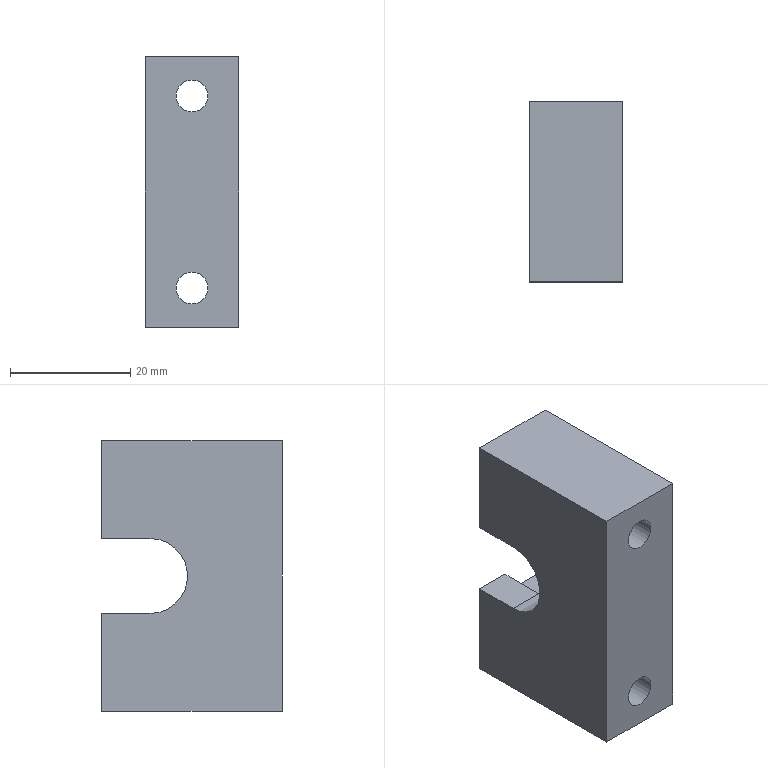Part | NX | 1 solid | 20 faces | box 15.5 x 30 x 45 mm | volume 14039 mm3 | plane 14 | cylinder 6 | commonest cylinder face diameters 5.3 x2 10 x2 12.5 x1 20 x1
STEP:
#1=CARTESIAN_POINT('',(6.,7.,-6.25));
#2=VERTEX_POINT('',#1);
#3=CARTESIAN_POINT('',(6.,7.,6.25));
#4=VERTEX_POINT('',#3);
#5=CARTESIAN_POINT('',(6.,7.,0.));
#6=DIRECTION('',(1.,0.,0.));
#7=DIRECTION('',(0.,0.,-1.));
#8=AXIS2_PLACEMENT_3D('',#5,#6,#7);
#9=CIRCLE('',#8,6.25);
#10=EDGE_CURVE('',#2,#4,#9,.F.);
#11=ORIENTED_EDGE('',*,*,#10,.F.);
#12=CARTESIAN_POINT('',(0.,7.,-6.25));
#13=VERTEX_POINT('',#12);
#14=CARTESIAN_POINT('',(-4.5,7.,-6.25));
#15=DIRECTION('',(1.,0.,0.));
#16=VECTOR('',#15,1000.);
#17=LINE('',#14,#16);
#18=EDGE_CURVE('',#13,#2,#17,.T.);
#19=ORIENTED_EDGE('',*,*,#18,.F.);
#20=CARTESIAN_POINT('',(0.,7.,6.25));
#21=VERTEX_POINT('',#20);
#22=CARTESIAN_POINT('',(0.,7.,0.));
#23=DIRECTION('',(1.,0.,0.));
#24=DIRECTION('',(0.,0.,-1.));
#25=AXIS2_PLACEMENT_3D('',#22,#23,#24);
#26=CIRCLE('',#25,6.25);
#27=EDGE_CURVE('',#21,#13,#26,.T.);
#28=ORIENTED_EDGE('',*,*,#27,.F.);
#29=CARTESIAN_POINT('',(-4.5,7.,6.25));
#30=DIRECTION('',(1.,0.,0.));
#31=VECTOR('',#30,1000.);
#32=LINE('',#29,#31);
#33=EDGE_CURVE('',#21,#4,#32,.T.);
#34=ORIENTED_EDGE('',*,*,#33,.T.);
#35=EDGE_LOOP('',(#11,#19,#28,#34));
#36=FACE_BOUND('',#35,.T.);
#37=CARTESIAN_POINT('',(-4.5,7.,0.));
#38=DIRECTION('',(1.,0.,0.));
#39=DIRECTION('',(0.,0.,-1.));
#40=AXIS2_PLACEMENT_3D('',#37,#38,#39);
#41=CYLINDRICAL_SURFACE('',#40,6.25);
#42=ADVANCED_FACE('',(#36),#41,.F.);
#43=CARTESIAN_POINT('',(6.,15.,6.25));
#44=VERTEX_POINT('',#43);
#45=CARTESIAN_POINT('',(6.,7.,6.25));
#46=DIRECTION('',(0.,1.,0.));
#47=VECTOR('',#46,1000.);
#48=LINE('',#45,#47);
#49=EDGE_CURVE('',#4,#44,#48,.T.);
#50=ORIENTED_EDGE('',*,*,#49,.F.);
#51=ORIENTED_EDGE('',*,*,#33,.F.);
#52=CARTESIAN_POINT('',(0.,15.,6.25));
#53=VERTEX_POINT('',#52);
#54=CARTESIAN_POINT('',(0.,0.,6.25));
#55=DIRECTION('',(0.,-1.,0.));
#56=VECTOR('',#55,1000.);
#57=LINE('',#54,#56);
#58=EDGE_CURVE('',#53,#21,#57,.T.);
#59=ORIENTED_EDGE('',*,*,#58,.F.);
#60=CARTESIAN_POINT('',(15.5,15.,6.25));
#61=DIRECTION('',(-1.,0.,0.));
#62=VECTOR('',#61,1000.);
#63=LINE('',#60,#62);
#64=EDGE_CURVE('',#44,#53,#63,.T.);
#65=ORIENTED_EDGE('',*,*,#64,.F.);
#66=EDGE_LOOP('',(#50,#51,#59,#65));
#67=FACE_BOUND('',#66,.T.);
#68=CARTESIAN_POINT('',(-4.5,7.,6.25));
#69=DIRECTION('',(0.,0.,1.));
#70=DIRECTION('',(0.,-1.,0.));
#71=AXIS2_PLACEMENT_3D('',#68,#69,#70);
#72=PLANE('',#71);
#73=ADVANCED_FACE('',(#67),#72,.F.);
#74=CARTESIAN_POINT('',(6.,15.,-6.25));
#75=VERTEX_POINT('',#74);
#76=CARTESIAN_POINT('',(6.,7.,-6.25));
#77=DIRECTION('',(0.,-1.,0.));
#78=VECTOR('',#77,1000.);
#79=LINE('',#76,#78);
#80=EDGE_CURVE('',#75,#2,#79,.T.);
#81=ORIENTED_EDGE('',*,*,#80,.F.);
#82=CARTESIAN_POINT('',(0.,15.,-6.25));
#83=VERTEX_POINT('',#82);
#84=CARTESIAN_POINT('',(15.5,15.,-6.25));
#85=DIRECTION('',(1.,0.,0.));
#86=VECTOR('',#85,1000.);
#87=LINE('',#84,#86);
#88=EDGE_CURVE('',#83,#75,#87,.T.);
#89=ORIENTED_EDGE('',*,*,#88,.F.);
#90=CARTESIAN_POINT('',(0.,0.,-6.25));
#91=DIRECTION('',(0.,1.,0.));
#92=VECTOR('',#91,1000.);
#93=LINE('',#90,#92);
#94=EDGE_CURVE('',#13,#83,#93,.T.);
#95=ORIENTED_EDGE('',*,*,#94,.F.);
#96=ORIENTED_EDGE('',*,*,#18,.T.);
#97=EDGE_LOOP('',(#81,#89,#95,#96));
#98=FACE_BOUND('',#97,.T.);
#99=CARTESIAN_POINT('',(-4.5,7.,-6.25));
#100=DIRECTION('',(0.,0.,-1.));
#101=DIRECTION('',(0.,1.,0.));
#102=AXIS2_PLACEMENT_3D('',#99,#100,#101);
#103=PLANE('',#102);
#104=ADVANCED_FACE('',(#98),#103,.F.);
#105=CARTESIAN_POINT('',(7.75,15.,21.));
#106=VERTEX_POINT('',#105);
#107=CARTESIAN_POINT('',(7.75,15.,16.));
#108=DIRECTION('',(0.,1.,0.));
#109=DIRECTION('',(0.,0.,1.));
#110=AXIS2_PLACEMENT_3D('',#107,#108,#109);
#111=CIRCLE('',#110,5.);
#112=EDGE_CURVE('',#106,#106,#111,.T.);
#113=ORIENTED_EDGE('',*,*,#112,.F.);
#114=EDGE_LOOP('',(#113));
#115=FACE_BOUND('',#114,.T.);
#116=CARTESIAN_POINT('',(15.5,15.,10.));
#117=VERTEX_POINT('',#116);
#118=CARTESIAN_POINT('',(15.5,15.,22.5));
#119=VERTEX_POINT('',#118);
#120=CARTESIAN_POINT('',(15.5,15.,22.5));
#121=DIRECTION('',(0.,0.,1.));
#122=VECTOR('',#121,1000.);
#123=LINE('',#120,#122);
#124=EDGE_CURVE('',#117,#119,#123,.T.);
#125=ORIENTED_EDGE('',*,*,#124,.F.);
#126=CARTESIAN_POINT('',(6.,15.,10.));
#127=VERTEX_POINT('',#126);
#128=CARTESIAN_POINT('',(6.,15.,10.));
#129=DIRECTION('',(1.,0.,0.));
#130=VECTOR('',#129,1000.);
#131=LINE('',#128,#130);
#132=EDGE_CURVE('',#127,#117,#131,.T.);
#133=ORIENTED_EDGE('',*,*,#132,.F.);
#134=CARTESIAN_POINT('',(6.,15.,22.5));
#135=DIRECTION('',(0.,0.,1.));
#136=VECTOR('',#135,1000.);
#137=LINE('',#134,#136);
#138=EDGE_CURVE('',#44,#127,#137,.T.);
#139=ORIENTED_EDGE('',*,*,#138,.F.);
#140=ORIENTED_EDGE('',*,*,#64,.T.);
#141=CARTESIAN_POINT('',(0.,15.,22.5));
#142=VERTEX_POINT('',#141);
#143=CARTESIAN_POINT('',(0.,15.,22.5));
#144=DIRECTION('',(0.,0.,1.));
#145=VECTOR('',#144,1000.);
#146=LINE('',#143,#145);
#147=EDGE_CURVE('',#53,#142,#146,.T.);
#148=ORIENTED_EDGE('',*,*,#147,.T.);
#149=CARTESIAN_POINT('',(15.5,15.,22.5));
#150=DIRECTION('',(-1.,0.,0.));
#151=VECTOR('',#150,1000.);
#152=LINE('',#149,#151);
#153=EDGE_CURVE('',#119,#142,#152,.T.);
#154=ORIENTED_EDGE('',*,*,#153,.F.);
#155=EDGE_LOOP('',(#125,#133,#139,#140,#148,#154));
#156=FACE_BOUND('',#155,.T.);
#157=CARTESIAN_POINT('',(15.5,15.,22.5));
#158=DIRECTION('',(0.,-1.,0.));
#159=DIRECTION('',(0.,0.,-1.));
#160=AXIS2_PLACEMENT_3D('',#157,#158,#159);
#161=PLANE('',#160);
#162=ADVANCED_FACE('',(#115,#156),#161,.F.);
#163=CARTESIAN_POINT('',(0.,-15.,-22.5));
#164=VERTEX_POINT('',#163);
#165=CARTESIAN_POINT('',(0.,15.,-22.5));
#166=VERTEX_POINT('',#165);
#167=CARTESIAN_POINT('',(0.,15.,-22.5));
#168=DIRECTION('',(0.,1.,0.));
#169=VECTOR('',#168,1000.);
#170=LINE('',#167,#169);
#171=EDGE_CURVE('',#164,#166,#170,.T.);
#172=ORIENTED_EDGE('',*,*,#171,.T.);
#173=CARTESIAN_POINT('',(15.5,15.,-22.5));
#174=VERTEX_POINT('',#173);
#175=CARTESIAN_POINT('',(15.5,15.,-22.5));
#176=DIRECTION('',(-1.,0.,0.));
#177=VECTOR('',#176,1000.);
#178=LINE('',#175,#177);
#179=EDGE_CURVE('',#174,#166,#178,.T.);
#180=ORIENTED_EDGE('',*,*,#179,.F.);
#181=CARTESIAN_POINT('',(15.5,-15.,-22.5));
#182=VERTEX_POINT('',#181);
#183=CARTESIAN_POINT('',(15.5,15.,-22.5));
#184=DIRECTION('',(0.,1.,0.));
#185=VECTOR('',#184,1000.);
#186=LINE('',#183,#185);
#187=EDGE_CURVE('',#182,#174,#186,.T.);
#188=ORIENTED_EDGE('',*,*,#187,.F.);
#189=CARTESIAN_POINT('',(15.5,-15.,-22.5));
#190=DIRECTION('',(-1.,0.,0.));
#191=VECTOR('',#190,1000.);
#192=LINE('',#189,#191);
#193=EDGE_CURVE('',#182,#164,#192,.T.);
#194=ORIENTED_EDGE('',*,*,#193,.T.);
#195=EDGE_LOOP('',(#172,#180,#188,#194));
#196=FACE_BOUND('',#195,.T.);
#197=CARTESIAN_POINT('',(15.5,15.,-22.5));
#198=DIRECTION('',(0.,0.,1.));
#199=DIRECTION('',(0.,-1.,0.));
#200=AXIS2_PLACEMENT_3D('',#197,#198,#199);
#201=PLANE('',#200);
#202=ADVANCED_FACE('',(#196),#201,.F.);
#203=CARTESIAN_POINT('',(7.75,15.,-11.));
#204=VERTEX_POINT('',#203);
#205=CARTESIAN_POINT('',(7.75,15.,-16.));
#206=DIRECTION('',(0.,1.,0.));
#207=DIRECTION('',(0.,0.,1.));
#208=AXIS2_PLACEMENT_3D('',#205,#206,#207);
#209=CIRCLE('',#208,5.);
#210=EDGE_CURVE('',#204,#204,#209,.T.);
#211=ORIENTED_EDGE('',*,*,#210,.F.);
#212=EDGE_LOOP('',(#211));
#213=FACE_BOUND('',#212,.T.);
#214=CARTESIAN_POINT('',(6.,15.,-10.));
#215=VERTEX_POINT('',#214);
#216=CARTESIAN_POINT('',(6.,15.,22.5));
#217=DIRECTION('',(0.,0.,1.));
#218=VECTOR('',#217,1000.);
#219=LINE('',#216,#218);
#220=EDGE_CURVE('',#215,#75,#219,.T.);
#221=ORIENTED_EDGE('',*,*,#220,.F.);
#222=CARTESIAN_POINT('',(15.5,15.,-10.));
#223=VERTEX_POINT('',#222);
#224=CARTESIAN_POINT('',(6.,15.,-10.));
#225=DIRECTION('',(1.,0.,0.));
#226=VECTOR('',#225,1000.);
#227=LINE('',#224,#226);
#228=EDGE_CURVE('',#215,#223,#227,.T.);
#229=ORIENTED_EDGE('',*,*,#228,.T.);
#230=CARTESIAN_POINT('',(15.5,15.,22.5));
#231=DIRECTION('',(0.,0.,1.));
#232=VECTOR('',#231,1000.);
#233=LINE('',#230,#232);
#234=EDGE_CURVE('',#174,#223,#233,.T.);
#235=ORIENTED_EDGE('',*,*,#234,.F.);
#236=ORIENTED_EDGE('',*,*,#179,.T.);
#237=CARTESIAN_POINT('',(0.,15.,22.5));
#238=DIRECTION('',(0.,0.,1.));
#239=VECTOR('',#238,1000.);
#240=LINE('',#237,#239);
#241=EDGE_CURVE('',#166,#83,#240,.T.);
#242=ORIENTED_EDGE('',*,*,#241,.T.);
#243=ORIENTED_EDGE('',*,*,#88,.T.);
#244=EDGE_LOOP('',(#221,#229,#235,#236,#242,#243));
#245=FACE_BOUND('',#244,.T.);
#246=CARTESIAN_POINT('',(15.5,15.,22.5));
#247=DIRECTION('',(0.,-1.,0.));
#248=DIRECTION('',(0.,0.,-1.));
#249=AXIS2_PLACEMENT_3D('',#246,#247,#248);
#250=PLANE('',#249);
#251=ADVANCED_FACE('',(#213,#245),#250,.F.);
#252=CARTESIAN_POINT('',(0.,-15.,22.5));
#253=VERTEX_POINT('',#252);
#254=CARTESIAN_POINT('',(0.,15.,22.5));
#255=DIRECTION('',(0.,-1.,0.));
#256=VECTOR('',#255,1000.);
#257=LINE('',#254,#256);
#258=EDGE_CURVE('',#142,#253,#257,.T.);
#259=ORIENTED_EDGE('',*,*,#258,.T.);
#260=CARTESIAN_POINT('',(15.5,-15.,22.5));
#261=VERTEX_POINT('',#260);
#262=CARTESIAN_POINT('',(15.5,-15.,22.5));
#263=DIRECTION('',(-1.,0.,0.));
#264=VECTOR('',#263,1000.);
#265=LINE('',#262,#264);
#266=EDGE_CURVE('',#261,#253,#265,.T.);
#267=ORIENTED_EDGE('',*,*,#266,.F.);
#268=CARTESIAN_POINT('',(15.5,15.,22.5));
#269=DIRECTION('',(0.,-1.,0.));
#270=VECTOR('',#269,1000.);
#271=LINE('',#268,#270);
#272=EDGE_CURVE('',#119,#261,#271,.T.);
#273=ORIENTED_EDGE('',*,*,#272,.F.);
#274=ORIENTED_EDGE('',*,*,#153,.T.);
#275=EDGE_LOOP('',(#259,#267,#273,#274));
#276=FACE_BOUND('',#275,.T.);
#277=CARTESIAN_POINT('',(15.5,15.,22.5));
#278=DIRECTION('',(0.,0.,-1.));
#279=DIRECTION('',(-1.,0.,0.));
#280=AXIS2_PLACEMENT_3D('',#277,#278,#279);
#281=PLANE('',#280);
#282=ADVANCED_FACE('',(#276),#281,.F.);
#283=CARTESIAN_POINT('',(7.75,-15.,-13.35));
#284=VERTEX_POINT('',#283);
#285=CARTESIAN_POINT('',(7.75,-15.,-16.));
#286=DIRECTION('',(0.,1.,0.));
#287=DIRECTION('',(0.,0.,1.));
#288=AXIS2_PLACEMENT_3D('',#285,#286,#287);
#289=CIRCLE('',#288,2.65);
#290=EDGE_CURVE('',#284,#284,#289,.T.);
#291=ORIENTED_EDGE('',*,*,#290,.T.);
#292=EDGE_LOOP('',(#291));
#293=FACE_BOUND('',#292,.T.);
#294=CARTESIAN_POINT('',(7.75,-15.,18.65));
#295=VERTEX_POINT('',#294);
#296=CARTESIAN_POINT('',(7.75,-15.,16.));
#297=DIRECTION('',(0.,1.,0.));
#298=DIRECTION('',(0.,0.,1.));
#299=AXIS2_PLACEMENT_3D('',#296,#297,#298);
#300=CIRCLE('',#299,2.65);
#301=EDGE_CURVE('',#295,#295,#300,.T.);
#302=ORIENTED_EDGE('',*,*,#301,.T.);
#303=EDGE_LOOP('',(#302));
#304=FACE_BOUND('',#303,.T.);
#305=CARTESIAN_POINT('',(0.,-15.,22.5));
#306=DIRECTION('',(0.,0.,-1.));
#307=VECTOR('',#306,1000.);
#308=LINE('',#305,#307);
#309=EDGE_CURVE('',#253,#164,#308,.T.);
#310=ORIENTED_EDGE('',*,*,#309,.T.);
#311=ORIENTED_EDGE('',*,*,#193,.F.);
#312=CARTESIAN_POINT('',(15.5,-15.,22.5));
#313=DIRECTION('',(0.,0.,-1.));
#314=VECTOR('',#313,1000.);
#315=LINE('',#312,#314);
#316=EDGE_CURVE('',#261,#182,#315,.T.);
#317=ORIENTED_EDGE('',*,*,#316,.F.);
#318=ORIENTED_EDGE('',*,*,#266,.T.);
#319=EDGE_LOOP('',(#310,#311,#317,#318));
#320=FACE_BOUND('',#319,.T.);
#321=CARTESIAN_POINT('',(15.5,-15.,22.5));
#322=DIRECTION('',(0.,1.,0.));
#323=DIRECTION('',(0.,0.,1.));
#324=AXIS2_PLACEMENT_3D('',#321,#322,#323);
#325=PLANE('',#324);
#326=ADVANCED_FACE('',(#293,#304,#320),#325,.F.);
#327=CARTESIAN_POINT('',(15.5,7.,10.));
#328=VERTEX_POINT('',#327);
#329=CARTESIAN_POINT('',(15.5,7.,10.));
#330=DIRECTION('',(0.,-1.,0.));
#331=VECTOR('',#330,1000.);
#332=LINE('',#329,#331);
#333=EDGE_CURVE('',#117,#328,#332,.T.);
#334=ORIENTED_EDGE('',*,*,#333,.F.);
#335=ORIENTED_EDGE('',*,*,#124,.T.);
#336=ORIENTED_EDGE('',*,*,#272,.T.);
#337=ORIENTED_EDGE('',*,*,#316,.T.);
#338=ORIENTED_EDGE('',*,*,#187,.T.);
#339=ORIENTED_EDGE('',*,*,#234,.T.);
#340=CARTESIAN_POINT('',(15.5,7.,-10.));
#341=VERTEX_POINT('',#340);
#342=CARTESIAN_POINT('',(15.5,7.,-10.));
#343=DIRECTION('',(0.,1.,0.));
#344=VECTOR('',#343,1000.);
#345=LINE('',#342,#344);
#346=EDGE_CURVE('',#341,#223,#345,.T.);
#347=ORIENTED_EDGE('',*,*,#346,.F.);
#348=CARTESIAN_POINT('',(15.5,7.,0.));
#349=DIRECTION('',(1.,0.,0.));
#350=DIRECTION('',(0.,0.,-1.));
#351=AXIS2_PLACEMENT_3D('',#348,#349,#350);
#352=CIRCLE('',#351,10.);
#353=EDGE_CURVE('',#328,#341,#352,.T.);
#354=ORIENTED_EDGE('',*,*,#353,.F.);
#355=EDGE_LOOP('',(#334,#335,#336,#337,#338,#339,#347,#354));
#356=FACE_BOUND('',#355,.T.);
#357=CARTESIAN_POINT('',(15.5,0.,0.));
#358=DIRECTION('',(1.,0.,0.));
#359=DIRECTION('',(0.,0.,-1.));
#360=AXIS2_PLACEMENT_3D('',#357,#358,#359);
#361=PLANE('',#360);
#362=ADVANCED_FACE('',(#356),#361,.T.);
#363=ORIENTED_EDGE('',*,*,#147,.F.);
#364=ORIENTED_EDGE('',*,*,#58,.T.);
#365=ORIENTED_EDGE('',*,*,#27,.T.);
#366=ORIENTED_EDGE('',*,*,#94,.T.);
#367=ORIENTED_EDGE('',*,*,#241,.F.);
#368=ORIENTED_EDGE('',*,*,#171,.F.);
#369=ORIENTED_EDGE('',*,*,#309,.F.);
#370=ORIENTED_EDGE('',*,*,#258,.F.);
#371=EDGE_LOOP('',(#363,#364,#365,#366,#367,#368,#369,#370));
#372=FACE_BOUND('',#371,.T.);
#373=CARTESIAN_POINT('',(0.,0.,0.));
#374=DIRECTION('',(1.,0.,0.));
#375=DIRECTION('',(0.,0.,-1.));
#376=AXIS2_PLACEMENT_3D('',#373,#374,#375);
#377=PLANE('',#376);
#378=ADVANCED_FACE('',(#372),#377,.F.);
#379=ORIENTED_EDGE('',*,*,#138,.T.);
#380=CARTESIAN_POINT('',(6.,7.,10.));
#381=VERTEX_POINT('',#380);
#382=CARTESIAN_POINT('',(6.,7.,10.));
#383=DIRECTION('',(0.,-1.,0.));
#384=VECTOR('',#383,1000.);
#385=LINE('',#382,#384);
#386=EDGE_CURVE('',#127,#381,#385,.T.);
#387=ORIENTED_EDGE('',*,*,#386,.T.);
#388=CARTESIAN_POINT('',(6.,7.,-10.));
#389=VERTEX_POINT('',#388);
#390=CARTESIAN_POINT('',(6.,7.,0.));
#391=DIRECTION('',(1.,0.,0.));
#392=DIRECTION('',(0.,0.,-1.));
#393=AXIS2_PLACEMENT_3D('',#390,#391,#392);
#394=CIRCLE('',#393,10.);
#395=EDGE_CURVE('',#381,#389,#394,.T.);
#396=ORIENTED_EDGE('',*,*,#395,.T.);
#397=CARTESIAN_POINT('',(6.,7.,-10.));
#398=DIRECTION('',(0.,1.,0.));
#399=VECTOR('',#398,1000.);
#400=LINE('',#397,#399);
#401=EDGE_CURVE('',#389,#215,#400,.T.);
#402=ORIENTED_EDGE('',*,*,#401,.T.);
#403=ORIENTED_EDGE('',*,*,#220,.T.);
#404=ORIENTED_EDGE('',*,*,#80,.T.);
#405=ORIENTED_EDGE('',*,*,#10,.T.);
#406=ORIENTED_EDGE('',*,*,#49,.T.);
#407=EDGE_LOOP('',(#379,#387,#396,#402,#403,#404,#405,#406));
#408=FACE_BOUND('',#407,.T.);
#409=CARTESIAN_POINT('',(6.,7.,0.));
#410=DIRECTION('',(1.,0.,0.));
#411=DIRECTION('',(0.,0.,-1.));
#412=AXIS2_PLACEMENT_3D('',#409,#410,#411);
#413=PLANE('',#412);
#414=ADVANCED_FACE('',(#408),#413,.T.);
#415=ORIENTED_EDGE('',*,*,#353,.T.);
#416=CARTESIAN_POINT('',(6.,7.,-10.));
#417=DIRECTION('',(1.,0.,0.));
#418=VECTOR('',#417,1000.);
#419=LINE('',#416,#418);
#420=EDGE_CURVE('',#389,#341,#419,.T.);
#421=ORIENTED_EDGE('',*,*,#420,.F.);
#422=ORIENTED_EDGE('',*,*,#395,.F.);
#423=CARTESIAN_POINT('',(6.,7.,10.));
#424=DIRECTION('',(1.,0.,0.));
#425=VECTOR('',#424,1000.);
#426=LINE('',#423,#425);
#427=EDGE_CURVE('',#381,#328,#426,.T.);
#428=ORIENTED_EDGE('',*,*,#427,.T.);
#429=EDGE_LOOP('',(#415,#421,#422,#428));
#430=FACE_BOUND('',#429,.T.);
#431=CARTESIAN_POINT('',(6.,7.,0.));
#432=DIRECTION('',(1.,0.,0.));
#433=DIRECTION('',(0.,0.,-1.));
#434=AXIS2_PLACEMENT_3D('',#431,#432,#433);
#435=CYLINDRICAL_SURFACE('',#434,10.);
#436=ADVANCED_FACE('',(#430),#435,.F.);
#437=ORIENTED_EDGE('',*,*,#333,.T.);
#438=ORIENTED_EDGE('',*,*,#427,.F.);
#439=ORIENTED_EDGE('',*,*,#386,.F.);
#440=ORIENTED_EDGE('',*,*,#132,.T.);
#441=EDGE_LOOP('',(#437,#438,#439,#440));
#442=FACE_BOUND('',#441,.T.);
#443=CARTESIAN_POINT('',(6.,7.,10.));
#444=DIRECTION('',(0.,0.,1.));
#445=DIRECTION('',(1.,0.,0.));
#446=AXIS2_PLACEMENT_3D('',#443,#444,#445);
#447=PLANE('',#446);
#448=ADVANCED_FACE('',(#442),#447,.F.);
#449=ORIENTED_EDGE('',*,*,#346,.T.);
#450=ORIENTED_EDGE('',*,*,#228,.F.);
#451=ORIENTED_EDGE('',*,*,#401,.F.);
#452=ORIENTED_EDGE('',*,*,#420,.T.);
#453=EDGE_LOOP('',(#449,#450,#451,#452));
#454=FACE_BOUND('',#453,.T.);
#455=CARTESIAN_POINT('',(6.,7.,-10.));
#456=DIRECTION('',(0.,0.,-1.));
#457=DIRECTION('',(-1.,0.,0.));
#458=AXIS2_PLACEMENT_3D('',#455,#456,#457);
#459=PLANE('',#458);
#460=ADVANCED_FACE('',(#454),#459,.F.);
#461=ORIENTED_EDGE('',*,*,#301,.F.);
#462=EDGE_LOOP('',(#461));
#463=FACE_BOUND('',#462,.T.);
#464=CARTESIAN_POINT('',(7.75,1.,18.65));
#465=VERTEX_POINT('',#464);
#466=CARTESIAN_POINT('',(7.75,1.,16.));
#467=DIRECTION('',(0.,1.,0.));
#468=DIRECTION('',(0.,0.,1.));
#469=AXIS2_PLACEMENT_3D('',#466,#467,#468);
#470=CIRCLE('',#469,2.65);
#471=EDGE_CURVE('',#465,#465,#470,.T.);
#472=ORIENTED_EDGE('',*,*,#471,.T.);
#473=EDGE_LOOP('',(#472));
#474=FACE_BOUND('',#473,.T.);
#475=CARTESIAN_POINT('',(7.75,15.,16.));
#476=DIRECTION('',(0.,1.,0.));
#477=DIRECTION('',(0.,0.,1.));
#478=AXIS2_PLACEMENT_3D('',#475,#476,#477);
#479=CYLINDRICAL_SURFACE('',#478,2.65);
#480=ADVANCED_FACE('',(#463,#474),#479,.F.);
#481=ORIENTED_EDGE('',*,*,#471,.F.);
#482=EDGE_LOOP('',(#481));
#483=FACE_BOUND('',#482,.T.);
#484=CARTESIAN_POINT('',(7.75,1.,21.));
#485=VERTEX_POINT('',#484);
#486=CARTESIAN_POINT('',(7.75,1.,16.));
#487=DIRECTION('',(0.,1.,0.));
#488=DIRECTION('',(0.,0.,1.));
#489=AXIS2_PLACEMENT_3D('',#486,#487,#488);
#490=CIRCLE('',#489,5.);
#491=EDGE_CURVE('',#485,#485,#490,.T.);
#492=ORIENTED_EDGE('',*,*,#491,.T.);
#493=EDGE_LOOP('',(#492));
#494=FACE_BOUND('',#493,.T.);
#495=CARTESIAN_POINT('',(10.4,1.,16.));
#496=DIRECTION('',(0.,-1.,0.));
#497=DIRECTION('',(0.,0.,-1.));
#498=AXIS2_PLACEMENT_3D('',#495,#496,#497);
#499=PLANE('',#498);
#500=ADVANCED_FACE('',(#483,#494),#499,.F.);
#501=ORIENTED_EDGE('',*,*,#491,.F.);
#502=EDGE_LOOP('',(#501));
#503=FACE_BOUND('',#502,.T.);
#504=ORIENTED_EDGE('',*,*,#112,.T.);
#505=EDGE_LOOP('',(#504));
#506=FACE_BOUND('',#505,.T.);
#507=CARTESIAN_POINT('',(7.75,15.,16.));
#508=DIRECTION('',(0.,1.,0.));
#509=DIRECTION('',(0.,0.,1.));
#510=AXIS2_PLACEMENT_3D('',#507,#508,#509);
#511=CYLINDRICAL_SURFACE('',#510,5.);
#512=ADVANCED_FACE('',(#503,#506),#511,.F.);
#513=ORIENTED_EDGE('',*,*,#290,.F.);
#514=EDGE_LOOP('',(#513));
#515=FACE_BOUND('',#514,.T.);
#516=CARTESIAN_POINT('',(7.75,1.,-13.35));
#517=VERTEX_POINT('',#516);
#518=CARTESIAN_POINT('',(7.75,1.,-16.));
#519=DIRECTION('',(0.,1.,0.));
#520=DIRECTION('',(0.,0.,1.));
#521=AXIS2_PLACEMENT_3D('',#518,#519,#520);
#522=CIRCLE('',#521,2.65);
#523=EDGE_CURVE('',#517,#517,#522,.T.);
#524=ORIENTED_EDGE('',*,*,#523,.T.);
#525=EDGE_LOOP('',(#524));
#526=FACE_BOUND('',#525,.T.);
#527=CARTESIAN_POINT('',(7.75,15.,-16.));
#528=DIRECTION('',(0.,1.,0.));
#529=DIRECTION('',(0.,0.,1.));
#530=AXIS2_PLACEMENT_3D('',#527,#528,#529);
#531=CYLINDRICAL_SURFACE('',#530,2.65);
#532=ADVANCED_FACE('',(#515,#526),#531,.F.);
#533=ORIENTED_EDGE('',*,*,#523,.F.);
#534=EDGE_LOOP('',(#533));
#535=FACE_BOUND('',#534,.T.);
#536=CARTESIAN_POINT('',(7.75,1.,-11.));
#537=VERTEX_POINT('',#536);
#538=CARTESIAN_POINT('',(7.75,1.,-16.));
#539=DIRECTION('',(0.,1.,0.));
#540=DIRECTION('',(0.,0.,1.));
#541=AXIS2_PLACEMENT_3D('',#538,#539,#540);
#542=CIRCLE('',#541,5.);
#543=EDGE_CURVE('',#537,#537,#542,.T.);
#544=ORIENTED_EDGE('',*,*,#543,.T.);
#545=EDGE_LOOP('',(#544));
#546=FACE_BOUND('',#545,.T.);
#547=CARTESIAN_POINT('',(10.4,1.,-16.));
#548=DIRECTION('',(0.,-1.,0.));
#549=DIRECTION('',(0.,0.,-1.));
#550=AXIS2_PLACEMENT_3D('',#547,#548,#549);
#551=PLANE('',#550);
#552=ADVANCED_FACE('',(#535,#546),#551,.F.);
#553=ORIENTED_EDGE('',*,*,#543,.F.);
#554=EDGE_LOOP('',(#553));
#555=FACE_BOUND('',#554,.T.);
#556=ORIENTED_EDGE('',*,*,#210,.T.);
#557=EDGE_LOOP('',(#556));
#558=FACE_BOUND('',#557,.T.);
#559=CARTESIAN_POINT('',(7.75,15.,-16.));
#560=DIRECTION('',(0.,1.,0.));
#561=DIRECTION('',(0.,0.,1.));
#562=AXIS2_PLACEMENT_3D('',#559,#560,#561);
#563=CYLINDRICAL_SURFACE('',#562,5.);
#564=ADVANCED_FACE('',(#555,#558),#563,.F.);
#565=CLOSED_SHELL('',(#42,#73,#104,#162,#202,#251,#282,#326,#362,#378,#414,#436,#448,#460,#480,#500,#512,#532,#552,#564));
#566=MANIFOLD_SOLID_BREP('',#565);
#567=(LENGTH_UNIT()NAMED_UNIT(*)SI_UNIT(.MILLI.,.METRE.));
#568=UNCERTAINTY_MEASURE_WITH_UNIT(LENGTH_MEASURE(0.00001),#567,'','');
#569=(NAMED_UNIT(*)PLANE_ANGLE_UNIT()SI_UNIT($,.RADIAN.));
#570=(NAMED_UNIT(*)SI_UNIT($,.STERADIAN.)SOLID_ANGLE_UNIT());
#571=(GEOMETRIC_REPRESENTATION_CONTEXT(3)GLOBAL_UNCERTAINTY_ASSIGNED_CONTEXT((#568))GLOBAL_UNIT_ASSIGNED_CONTEXT((#567,#569,#570))REPRESENTATION_CONTEXT('',''));
#572=ADVANCED_BREP_SHAPE_REPRESENTATION('',(#566),#571);